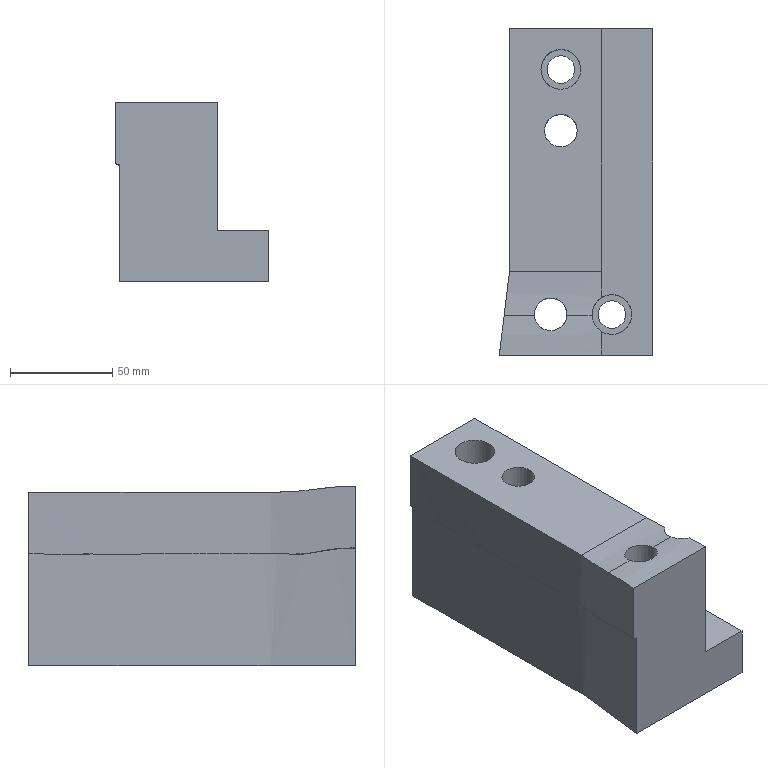Part | NX | features solid 2 | 1 solid | 21 faces | box 75.161 x 160 x 88.078 mm | volume 639767 mm3 | plane 9 | spline 6 | cylinder 6 | commonest cylinder face diameters 13.5 x2 16 x2 19.5 x2
STEP:
#1=CARTESIAN_POINT('',(-305.,78.37,-10.));
#2=VERTEX_POINT('',#1);
#3=CARTESIAN_POINT('',(-305.,78.37,50.536));
#4=VERTEX_POINT('',#3);
#5=CARTESIAN_POINT('',(-305.,78.37,-20.));
#6=DIRECTION('',(0.,0.,1.));
#7=VECTOR('',#6,1000.);
#8=LINE('',#5,#7);
#9=EDGE_CURVE('',#2,#4,#8,.T.);
#10=ORIENTED_EDGE('',*,*,#9,.F.);
#11=CARTESIAN_POINT('',(-305.,210.,-10.));
#12=VERTEX_POINT('',#11);
#13=CARTESIAN_POINT('',(-305.,315.,-10.));
#14=DIRECTION('',(0.,-1.,0.));
#15=VECTOR('',#14,1000.);
#16=LINE('',#13,#15);
#17=EDGE_CURVE('',#2,#12,#16,.F.);
#18=ORIENTED_EDGE('',*,*,#17,.T.);
#19=CARTESIAN_POINT('',(-305.,210.,50.));
#20=VERTEX_POINT('',#19);
#21=CARTESIAN_POINT('',(-305.,210.,-500.));
#22=DIRECTION('',(0.,0.,1.));
#23=VECTOR('',#22,1000.);
#24=LINE('',#21,#23);
#25=EDGE_CURVE('',#12,#20,#24,.T.);
#26=ORIENTED_EDGE('',*,*,#25,.T.);
#27=CARTESIAN_POINT('',(-305.,91.041,50.));
#28=VERTEX_POINT('',#27);
#29=CARTESIAN_POINT('',(-305.,91.041,50.));
#30=CARTESIAN_POINT('',(-305.,130.694,50.));
#31=CARTESIAN_POINT('',(-305.,170.347,50.));
#32=CARTESIAN_POINT('',(-305.,210.,50.));
#33=B_SPLINE_CURVE_WITH_KNOTS('',3,(#29,#30,#31,#32),.UNSPECIFIED.,.F.,.F.,(4,4),(0.,0.119),.UNSPECIFIED.);
#34=EDGE_CURVE('',#28,#20,#33,.T.);
#35=ORIENTED_EDGE('',*,*,#34,.F.);
#36=CARTESIAN_POINT('',(-305.,91.041,50.));
#37=CARTESIAN_POINT('',(-305.,86.812,50.));
#38=CARTESIAN_POINT('',(-305.,82.583,50.179));
#39=CARTESIAN_POINT('',(-305.,78.37,50.536));
#40=B_SPLINE_CURVE_WITH_KNOTS('',3,(#36,#37,#38,#39),.UNSPECIFIED.,.F.,.F.,(4,4),(0.,0.01269),.UNSPECIFIED.);
#41=EDGE_CURVE('',#28,#4,#40,.T.);
#42=ORIENTED_EDGE('',*,*,#41,.T.);
#43=EDGE_LOOP('',(#10,#18,#26,#35,#42));
#44=FACE_BOUND('',#43,.T.);
#45=CARTESIAN_POINT('',(-305.,340.,500.));
#46=DIRECTION('',(1.,0.,0.));
#47=DIRECTION('',(0.,0.,-1.));
#48=AXIS2_PLACEMENT_3D('',#45,#46,#47);
#49=PLANE('',#48);
#50=ADVANCED_FACE('',(#44),#49,.T.);
#51=CARTESIAN_POINT('',(-305.,61.63,52.478));
#52=VERTEX_POINT('',#51);
#53=CARTESIAN_POINT('',(-305.,61.63,-10.));
#54=VERTEX_POINT('',#53);
#55=CARTESIAN_POINT('',(-305.,61.63,-20.));
#56=DIRECTION('',(0.,0.,1.));
#57=VECTOR('',#56,1000.);
#58=LINE('',#55,#57);
#59=EDGE_CURVE('',#52,#54,#58,.F.);
#60=ORIENTED_EDGE('',*,*,#59,.F.);
#61=CARTESIAN_POINT('',(-305.,50.,53.078));
#62=VERTEX_POINT('',#61);
#63=CARTESIAN_POINT('',(-305.,50.,53.078));
#64=CARTESIAN_POINT('',(-305.,53.888,53.029));
#65=CARTESIAN_POINT('',(-305.,57.765,52.828));
#66=CARTESIAN_POINT('',(-305.,61.63,52.478));
#67=B_SPLINE_CURVE_WITH_KNOTS('',3,(#63,#64,#65,#66),.UNSPECIFIED.,.F.,.F.,(4,4),(0.,0.01164),.UNSPECIFIED.);
#68=EDGE_CURVE('',#62,#52,#67,.T.);
#69=ORIENTED_EDGE('',*,*,#68,.F.);
#70=CARTESIAN_POINT('',(-305.,50.,-10.));
#71=VERTEX_POINT('',#70);
#72=CARTESIAN_POINT('',(-305.,50.,-500.));
#73=DIRECTION('',(0.,0.,1.));
#74=VECTOR('',#73,1000.);
#75=LINE('',#72,#74);
#76=EDGE_CURVE('',#71,#62,#75,.T.);
#77=ORIENTED_EDGE('',*,*,#76,.F.);
#78=CARTESIAN_POINT('',(-305.,315.,-10.));
#79=DIRECTION('',(0.,-1.,0.));
#80=VECTOR('',#79,1000.);
#81=LINE('',#78,#80);
#82=EDGE_CURVE('',#71,#54,#81,.F.);
#83=ORIENTED_EDGE('',*,*,#82,.T.);
#84=EDGE_LOOP('',(#60,#69,#77,#83));
#85=FACE_BOUND('',#84,.T.);
#86=CARTESIAN_POINT('',(-305.,340.,500.));
#87=DIRECTION('',(1.,0.,0.));
#88=DIRECTION('',(0.,0.,-1.));
#89=AXIS2_PLACEMENT_3D('',#86,#87,#88);
#90=PLANE('',#89);
#91=ADVANCED_FACE('',(#85),#90,.T.);
#92=CARTESIAN_POINT('',(-353.138,50.,-35.));
#93=VERTEX_POINT('',#92);
#94=CARTESIAN_POINT('',(-280.,50.,-35.));
#95=VERTEX_POINT('',#94);
#96=CARTESIAN_POINT('',(-353.136,50.,-35.));
#97=DIRECTION('',(1.,0.,0.));
#98=VECTOR('',#97,1000.);
#99=LINE('',#96,#98);
#100=EDGE_CURVE('',#93,#95,#99,.T.);
#101=ORIENTED_EDGE('',*,*,#100,.T.);
#102=CARTESIAN_POINT('',(-280.,50.,-10.));
#103=VERTEX_POINT('',#102);
#104=CARTESIAN_POINT('',(-280.,50.,-500.));
#105=DIRECTION('',(0.,0.,1.));
#106=VECTOR('',#105,1000.);
#107=LINE('',#104,#106);
#108=EDGE_CURVE('',#95,#103,#107,.T.);
#109=ORIENTED_EDGE('',*,*,#108,.T.);
#110=CARTESIAN_POINT('',(365.,50.,-10.));
#111=DIRECTION('',(-1.,0.,0.));
#112=VECTOR('',#111,1000.);
#113=LINE('',#110,#112);
#114=EDGE_CURVE('',#71,#103,#113,.F.);
#115=ORIENTED_EDGE('',*,*,#114,.F.);
#116=ORIENTED_EDGE('',*,*,#76,.T.);
#117=CARTESIAN_POINT('',(-355.161,50.,53.078));
#118=VERTEX_POINT('',#117);
#119=CARTESIAN_POINT('',(-355.161,50.,53.078));
#120=CARTESIAN_POINT('',(-338.441,50.,53.078));
#121=CARTESIAN_POINT('',(-321.72,50.,53.078));
#122=CARTESIAN_POINT('',(-305.,50.,53.078));
#123=B_SPLINE_CURVE_WITH_KNOTS('',3,(#119,#120,#121,#122),.UNSPECIFIED.,.F.,.F.,(4,4),(0.00388,0.05404),.UNSPECIFIED.);
#124=EDGE_CURVE('',#118,#62,#123,.T.);
#125=ORIENTED_EDGE('',*,*,#124,.F.);
#126=CARTESIAN_POINT('',(-355.161,50.,22.792));
#127=VERTEX_POINT('',#126);
#128=CARTESIAN_POINT('',(-355.161,50.,37.356));
#129=DIRECTION('',(0.,0.,-1.));
#130=VECTOR('',#129,1000.);
#131=LINE('',#128,#130);
#132=EDGE_CURVE('',#118,#127,#131,.T.);
#133=ORIENTED_EDGE('',*,*,#132,.T.);
#134=CARTESIAN_POINT('',(-353.138,50.,22.67));
#135=VERTEX_POINT('',#134);
#136=CARTESIAN_POINT('',(-353.138,50.,22.67));
#137=CARTESIAN_POINT('',(-353.814,50.,22.701));
#138=CARTESIAN_POINT('',(-354.488,50.,22.741));
#139=CARTESIAN_POINT('',(-355.161,50.,22.792));
#140=B_SPLINE_CURVE_WITH_KNOTS('',3,(#136,#137,#138,#139),.UNSPECIFIED.,.F.,.F.,(4,4),(0.01465,0.01669),.UNSPECIFIED.);
#141=EDGE_CURVE('',#135,#127,#140,.T.);
#142=ORIENTED_EDGE('',*,*,#141,.F.);
#143=CARTESIAN_POINT('',(-353.138,50.,-84.379));
#144=DIRECTION('',(0.,0.,-1.));
#145=VECTOR('',#144,1000.);
#146=LINE('',#143,#145);
#147=EDGE_CURVE('',#93,#135,#146,.F.);
#148=ORIENTED_EDGE('',*,*,#147,.F.);
#149=EDGE_LOOP('',(#101,#109,#115,#116,#125,#133,#142,#148));
#150=FACE_BOUND('',#149,.T.);
#151=CARTESIAN_POINT('',(-353.136,50.,-500.));
#152=DIRECTION('',(0.,-1.,0.));
#153=DIRECTION('',(0.,0.,-1.));
#154=AXIS2_PLACEMENT_3D('',#151,#152,#153);
#155=PLANE('',#154);
#156=ADVANCED_FACE('',(#150),#155,.T.);
#157=ORIENTED_EDGE('',*,*,#25,.F.);
#158=CARTESIAN_POINT('',(-280.,210.,-10.));
#159=VERTEX_POINT('',#158);
#160=CARTESIAN_POINT('',(365.,210.,-10.));
#161=DIRECTION('',(-1.,0.,0.));
#162=VECTOR('',#161,1000.);
#163=LINE('',#160,#162);
#164=EDGE_CURVE('',#12,#159,#163,.F.);
#165=ORIENTED_EDGE('',*,*,#164,.T.);
#166=CARTESIAN_POINT('',(-280.,210.,-35.));
#167=VERTEX_POINT('',#166);
#168=CARTESIAN_POINT('',(-280.,210.,-500.));
#169=DIRECTION('',(0.,0.,1.));
#170=VECTOR('',#169,1000.);
#171=LINE('',#168,#170);
#172=EDGE_CURVE('',#167,#159,#171,.T.);
#173=ORIENTED_EDGE('',*,*,#172,.F.);
#174=CARTESIAN_POINT('',(-347.967,210.,-35.));
#175=VERTEX_POINT('',#174);
#176=CARTESIAN_POINT('',(-350.,210.,-35.));
#177=DIRECTION('',(1.,0.,0.));
#178=VECTOR('',#177,1000.);
#179=LINE('',#176,#178);
#180=EDGE_CURVE('',#175,#167,#179,.T.);
#181=ORIENTED_EDGE('',*,*,#180,.F.);
#182=CARTESIAN_POINT('',(-347.967,210.,19.922));
#183=VERTEX_POINT('',#182);
#184=CARTESIAN_POINT('',(-347.967,210.,-84.379));
#185=DIRECTION('',(0.,0.,-1.));
#186=VECTOR('',#185,1000.);
#187=LINE('',#184,#186);
#188=EDGE_CURVE('',#175,#183,#187,.F.);
#189=ORIENTED_EDGE('',*,*,#188,.T.);
#190=CARTESIAN_POINT('',(-349.967,210.,19.959));
#191=VERTEX_POINT('',#190);
#192=CARTESIAN_POINT('',(-347.967,210.,19.922));
#193=CARTESIAN_POINT('',(-348.633,210.,19.931));
#194=CARTESIAN_POINT('',(-349.3,210.,19.943));
#195=CARTESIAN_POINT('',(-349.967,210.,19.959));
#196=B_SPLINE_CURVE_WITH_KNOTS('',3,(#192,#193,#194,#195),.UNSPECIFIED.,.F.,.F.,(4,4),(0.004977,0.006977),.UNSPECIFIED.);
#197=EDGE_CURVE('',#183,#191,#196,.T.);
#198=ORIENTED_EDGE('',*,*,#197,.T.);
#199=CARTESIAN_POINT('',(-349.967,210.,50.));
#200=VERTEX_POINT('',#199);
#201=CARTESIAN_POINT('',(-349.967,210.,37.356));
#202=DIRECTION('',(0.,0.,-1.));
#203=VECTOR('',#202,1000.);
#204=LINE('',#201,#203);
#205=EDGE_CURVE('',#200,#191,#204,.T.);
#206=ORIENTED_EDGE('',*,*,#205,.F.);
#207=CARTESIAN_POINT('',(-265.,210.,50.));
#208=DIRECTION('',(1.,0.,0.));
#209=VECTOR('',#208,1000.);
#210=LINE('',#207,#209);
#211=EDGE_CURVE('',#200,#20,#210,.T.);
#212=ORIENTED_EDGE('',*,*,#211,.T.);
#213=EDGE_LOOP('',(#157,#165,#173,#181,#189,#198,#206,#212));
#214=FACE_BOUND('',#213,.T.);
#215=CARTESIAN_POINT('',(-350.,210.,-500.));
#216=DIRECTION('',(0.,-1.,0.));
#217=DIRECTION('',(0.,0.,-1.));
#218=AXIS2_PLACEMENT_3D('',#215,#216,#217);
#219=PLANE('',#218);
#220=ADVANCED_FACE('',(#214),#219,.F.);
#221=CARTESIAN_POINT('',(-337.988,69.567,51.545));
#222=VERTEX_POINT('',#221);
#223=CARTESIAN_POINT('',(-352.757,69.567,51.545));
#224=VERTEX_POINT('',#223);
#225=CARTESIAN_POINT('',(-337.988,69.567,51.545));
#226=CARTESIAN_POINT('',(-342.911,69.567,51.545));
#227=CARTESIAN_POINT('',(-347.834,69.567,51.545));
#228=CARTESIAN_POINT('',(-352.757,69.567,51.545));
#229=B_SPLINE_CURVE_WITH_KNOTS('',3,(#225,#226,#227,#228),.UNSPECIFIED.,.F.,.F.,(4,4),(0.9517,0.9933),.UNSPECIFIED.);
#230=EDGE_CURVE('',#222,#224,#229,.T.);
#231=ORIENTED_EDGE('',*,*,#230,.F.);
#232=CARTESIAN_POINT('',(-322.012,69.567,51.545));
#233=VERTEX_POINT('',#232);
#234=CARTESIAN_POINT('',(-337.988,69.567,51.545));
#235=CARTESIAN_POINT('',(-338.106,71.736,51.231));
#236=CARTESIAN_POINT('',(-336.503,76.106,50.718));
#237=CARTESIAN_POINT('',(-330.012,78.945,50.493));
#238=CARTESIAN_POINT('',(-323.498,76.115,50.717));
#239=CARTESIAN_POINT('',(-321.894,71.736,51.231));
#240=CARTESIAN_POINT('',(-322.012,69.567,51.545));
#241=B_SPLINE_CURVE_WITH_KNOTS('',3,(#234,#235,#236,#237,#238,#239,#240),.UNSPECIFIED.,.F.,.F.,(4,1,1,1,4),(0.,0.006491,0.01298,0.01947,0.02596),.UNSPECIFIED.);
#242=EDGE_CURVE('',#222,#233,#241,.T.);
#243=ORIENTED_EDGE('',*,*,#242,.T.);
#244=CARTESIAN_POINT('',(-309.74,69.567,51.545));
#245=VERTEX_POINT('',#244);
#246=CARTESIAN_POINT('',(-309.74,69.567,51.545));
#247=CARTESIAN_POINT('',(-313.831,69.567,51.545));
#248=CARTESIAN_POINT('',(-317.921,69.567,51.545));
#249=CARTESIAN_POINT('',(-322.012,69.567,51.545));
#250=B_SPLINE_CURVE_WITH_KNOTS('',3,(#246,#247,#248,#249),.UNSPECIFIED.,.F.,.F.,(4,4),(0.8721,0.9067),.UNSPECIFIED.);
#251=EDGE_CURVE('',#245,#233,#250,.T.);
#252=ORIENTED_EDGE('',*,*,#251,.F.);
#253=CARTESIAN_POINT('',(-309.74,69.567,51.545));
#254=CARTESIAN_POINT('',(-309.896,73.076,51.038));
#255=CARTESIAN_POINT('',(-308.044,76.552,50.69));
#256=CARTESIAN_POINT('',(-305.,78.37,50.536));
#257=B_SPLINE_CURVE_WITH_KNOTS('',3,(#253,#254,#255,#256),.UNSPECIFIED.,.F.,.F.,(4,4),(0.,0.0105),.UNSPECIFIED.);
#258=EDGE_CURVE('',#245,#4,#257,.T.);
#259=ORIENTED_EDGE('',*,*,#258,.T.);
#260=ORIENTED_EDGE('',*,*,#41,.F.);
#261=CARTESIAN_POINT('',(-350.144,91.041,50.));
#262=VERTEX_POINT('',#261);
#263=CARTESIAN_POINT('',(-350.144,91.041,50.));
#264=CARTESIAN_POINT('',(-335.096,91.041,50.));
#265=CARTESIAN_POINT('',(-320.048,91.041,50.));
#266=CARTESIAN_POINT('',(-305.,91.041,50.));
#267=B_SPLINE_CURVE_WITH_KNOTS('',3,(#263,#264,#265,#266),.UNSPECIFIED.,.F.,.F.,(4,4),(0.03072,0.3146),.UNSPECIFIED.);
#268=EDGE_CURVE('',#262,#28,#267,.T.);
#269=ORIENTED_EDGE('',*,*,#268,.F.);
#270=CARTESIAN_POINT('',(-350.144,91.041,50.));
#271=CARTESIAN_POINT('',(-350.286,89.236,50.));
#272=CARTESIAN_POINT('',(-350.787,85.654,50.065));
#273=CARTESIAN_POINT('',(-351.671,78.483,50.451));
#274=CARTESIAN_POINT('',(-352.321,73.122,51.031));
#275=CARTESIAN_POINT('',(-352.757,69.567,51.545));
#276=B_SPLINE_CURVE_WITH_KNOTS('',3,(#270,#271,#272,#273,#274,#275),.UNSPECIFIED.,.F.,.F.,(4,1,1,4),(0.,0.005425,0.01085,0.0217),.UNSPECIFIED.);
#277=EDGE_CURVE('',#262,#224,#276,.T.);
#278=ORIENTED_EDGE('',*,*,#277,.T.);
#279=EDGE_LOOP('',(#231,#243,#252,#259,#260,#269,#278));
#280=FACE_BOUND('',#279,.T.);
#281=CARTESIAN_POINT('',(-305.,69.567,51.545));
#282=CARTESIAN_POINT('',(-305.,80.248,50.));
#283=CARTESIAN_POINT('',(-305.,91.041,50.));
#284=CARTESIAN_POINT('',(-321.014,69.567,51.545));
#285=CARTESIAN_POINT('',(-321.014,80.248,50.));
#286=CARTESIAN_POINT('',(-321.014,91.041,50.));
#287=CARTESIAN_POINT('',(-337.029,69.567,51.545));
#288=CARTESIAN_POINT('',(-337.029,80.248,50.));
#289=CARTESIAN_POINT('',(-337.029,91.041,50.));
#290=CARTESIAN_POINT('',(-353.043,69.567,51.545));
#291=CARTESIAN_POINT('',(-353.043,80.248,50.));
#292=CARTESIAN_POINT('',(-353.043,91.041,50.));
#293=(BOUNDED_SURFACE()B_SPLINE_SURFACE(3,2,((#281,#282,#283),(#284,#285,#286),(#287,#288,#289),(#290,#291,#292)),.UNSPECIFIED.,.F.,.F.,.F.)B_SPLINE_SURFACE_WITH_KNOTS((4,4),(3,3),(0.8537,0.9881),(0.,1.),.PIECEWISE_BEZIER_KNOTS.)GEOMETRIC_REPRESENTATION_ITEM()RATIONAL_B_SPLINE_SURFACE(((1.,0.9974,1.),(1.,0.9974,1.),(1.,0.9974,1.),(1.,0.9974,1.)))REPRESENTATION_ITEM('')SURFACE());
#294=ADVANCED_FACE('',(#280),#293,.F.);
#295=CARTESIAN_POINT('',(-317.,160.,50.));
#296=VERTEX_POINT('',#295);
#297=CARTESIAN_POINT('',(-318.736,153.724,50.));
#298=CARTESIAN_POINT('',(-316.133,160.002,50.));
#299=CARTESIAN_POINT('',(-318.734,166.27,50.));
#300=CARTESIAN_POINT('',(-324.994,168.864,50.));
#301=CARTESIAN_POINT('',(-331.266,166.273,50.));
#302=CARTESIAN_POINT('',(-333.865,160.001,50.));
#303=CARTESIAN_POINT('',(-331.275,153.739,50.));
#304=CARTESIAN_POINT('',(-325.01,151.134,50.));
#305=CARTESIAN_POINT('',(-318.736,153.724,50.));
#306=CARTESIAN_POINT('',(-316.133,160.002,50.));
#307=CARTESIAN_POINT('',(-318.734,166.27,50.));
#308=B_SPLINE_CURVE_WITH_KNOTS('',3,(#297,#298,#299,#300,#301,#302,#303,#304,#305,#306,#307),.UNSPECIFIED.,.T.,.F.,(1,1,1,1,1,1,1,1,1,1,1,1,1,1,1),(-0.01876,-0.0125,-0.006252,0.,0.006252,0.0125,0.01876,0.02501,0.03126,0.03751,0.04377,0.05002,0.05627,0.06252,0.06877),.UNSPECIFIED.);
#309=EDGE_CURVE('',#296,#296,#308,.T.);
#310=ORIENTED_EDGE('',*,*,#309,.F.);
#311=EDGE_LOOP('',(#310));
#312=FACE_BOUND('',#311,.T.);
#313=CARTESIAN_POINT('',(-315.25,190.,50.));
#314=VERTEX_POINT('',#313);
#315=CARTESIAN_POINT('',(-317.366,182.351,50.));
#316=CARTESIAN_POINT('',(-314.193,190.002,50.));
#317=CARTESIAN_POINT('',(-317.363,197.641,50.));
#318=CARTESIAN_POINT('',(-324.992,200.803,50.));
#319=CARTESIAN_POINT('',(-332.637,197.646,50.));
#320=CARTESIAN_POINT('',(-335.804,190.001,50.));
#321=CARTESIAN_POINT('',(-332.648,182.37,50.));
#322=CARTESIAN_POINT('',(-325.012,179.195,50.));
#323=CARTESIAN_POINT('',(-317.366,182.351,50.));
#324=CARTESIAN_POINT('',(-314.193,190.002,50.));
#325=CARTESIAN_POINT('',(-317.363,197.641,50.));
#326=B_SPLINE_CURVE_WITH_KNOTS('',3,(#315,#316,#317,#318,#319,#320,#321,#322,#323,#324,#325),.UNSPECIFIED.,.T.,.F.,(1,1,1,1,1,1,1,1,1,1,1,1,1,1,1),(-0.02286,-0.01524,-0.00762,0.,0.00762,0.01524,0.02286,0.03048,0.0381,0.04572,0.05334,0.06096,0.06858,0.0762,0.08382),.UNSPECIFIED.);
#327=EDGE_CURVE('',#314,#314,#326,.T.);
#328=ORIENTED_EDGE('',*,*,#327,.F.);
#329=EDGE_LOOP('',(#328));
#330=FACE_BOUND('',#329,.T.);
#331=ORIENTED_EDGE('',*,*,#268,.T.);
#332=ORIENTED_EDGE('',*,*,#34,.T.);
#333=ORIENTED_EDGE('',*,*,#211,.F.);
#334=CARTESIAN_POINT('',(-350.144,91.041,50.));
#335=CARTESIAN_POINT('',(-349.948,93.519,50.));
#336=CARTESIAN_POINT('',(-350.035,98.476,50.));
#337=CARTESIAN_POINT('',(-350.015,105.911,50.));
#338=CARTESIAN_POINT('',(-350.022,113.346,50.));
#339=CARTESIAN_POINT('',(-350.007,123.259,50.));
#340=CARTESIAN_POINT('',(-350.002,135.65,50.));
#341=CARTESIAN_POINT('',(-349.996,155.476,50.));
#342=CARTESIAN_POINT('',(-350.034,180.259,50.));
#343=CARTESIAN_POINT('',(-349.982,200.087,50.));
#344=CARTESIAN_POINT('',(-349.967,210.,50.));
#345=B_SPLINE_CURVE_WITH_KNOTS('',3,(#334,#335,#336,#337,#338,#339,#340,#341,#342,#343,#344),.UNSPECIFIED.,.F.,.F.,(4,1,1,1,1,1,1,1,4),(0.,0.007435,0.01487,0.0223,0.02974,0.04461,0.05948,0.08922,0.119),.UNSPECIFIED.);
#346=EDGE_CURVE('',#262,#200,#345,.T.);
#347=ORIENTED_EDGE('',*,*,#346,.F.);
#348=EDGE_LOOP('',(#331,#332,#333,#347));
#349=FACE_BOUND('',#348,.T.);
#350=CARTESIAN_POINT('',(-305.,91.041,50.));
#351=CARTESIAN_POINT('',(-350.415,91.041,50.));
#352=CARTESIAN_POINT('',(-305.,210.,50.));
#353=CARTESIAN_POINT('',(-350.415,210.,50.));
#354=B_SPLINE_SURFACE_WITH_KNOTS('',1,1,((#350,#351),(#352,#353)),.PLANE_SURF.,.F.,.F.,.F.,(2,2),(2,2),(0.,0.471),(0.5755,0.6612),.PIECEWISE_BEZIER_KNOTS.);
#355=ADVANCED_FACE('',(#312,#330,#349),#354,.T.);
#356=CARTESIAN_POINT('',(-337.988,69.567,51.545));
#357=CARTESIAN_POINT('',(-337.878,67.542,51.838));
#358=CARTESIAN_POINT('',(-336.073,63.634,52.304));
#359=CARTESIAN_POINT('',(-330.001,61.184,52.514));
#360=CARTESIAN_POINT('',(-323.928,63.632,52.304));
#361=CARTESIAN_POINT('',(-322.122,67.542,51.838));
#362=CARTESIAN_POINT('',(-322.012,69.567,51.545));
#363=B_SPLINE_CURVE_WITH_KNOTS('',3,(#356,#357,#358,#359,#360,#361,#362),.UNSPECIFIED.,.F.,.F.,(4,1,1,1,4),(0.,0.00606,0.01212,0.01818,0.02424),.UNSPECIFIED.);
#364=EDGE_CURVE('',#222,#233,#363,.T.);
#365=ORIENTED_EDGE('',*,*,#364,.F.);
#366=ORIENTED_EDGE('',*,*,#230,.T.);
#367=CARTESIAN_POINT('',(-355.161,50.,53.078));
#368=CARTESIAN_POINT('',(-354.357,56.548,52.995));
#369=CARTESIAN_POINT('',(-353.553,63.081,52.483));
#370=CARTESIAN_POINT('',(-352.757,69.567,51.545));
#371=B_SPLINE_CURVE_WITH_KNOTS('',3,(#367,#368,#369,#370),.UNSPECIFIED.,.F.,.F.,(4,4),(0.02067,0.04046),.UNSPECIFIED.);
#372=EDGE_CURVE('',#118,#224,#371,.T.);
#373=ORIENTED_EDGE('',*,*,#372,.F.);
#374=ORIENTED_EDGE('',*,*,#124,.T.);
#375=ORIENTED_EDGE('',*,*,#68,.T.);
#376=CARTESIAN_POINT('',(-309.74,69.567,51.545));
#377=CARTESIAN_POINT('',(-309.597,66.347,52.011));
#378=CARTESIAN_POINT('',(-307.793,63.298,52.327));
#379=CARTESIAN_POINT('',(-305.,61.63,52.478));
#380=B_SPLINE_CURVE_WITH_KNOTS('',3,(#376,#377,#378,#379),.UNSPECIFIED.,.F.,.F.,(4,4),(0.,0.009631),.UNSPECIFIED.);
#381=EDGE_CURVE('',#245,#52,#380,.T.);
#382=ORIENTED_EDGE('',*,*,#381,.F.);
#383=ORIENTED_EDGE('',*,*,#251,.T.);
#384=EDGE_LOOP('',(#365,#366,#373,#374,#375,#382,#383));
#385=FACE_BOUND('',#384,.T.);
#386=CARTESIAN_POINT('',(-305.,69.567,51.545));
#387=CARTESIAN_POINT('',(-305.,59.775,52.962));
#388=CARTESIAN_POINT('',(-305.,49.882,53.08));
#389=CARTESIAN_POINT('',(-321.821,69.567,51.545));
#390=CARTESIAN_POINT('',(-321.821,59.775,52.962));
#391=CARTESIAN_POINT('',(-321.821,49.882,53.08));
#392=CARTESIAN_POINT('',(-338.641,69.567,51.545));
#393=CARTESIAN_POINT('',(-338.641,59.775,52.962));
#394=CARTESIAN_POINT('',(-338.641,49.882,53.08));
#395=CARTESIAN_POINT('',(-355.462,69.567,51.545));
#396=CARTESIAN_POINT('',(-355.462,59.775,52.962));
#397=CARTESIAN_POINT('',(-355.462,49.882,53.08));
#398=(BOUNDED_SURFACE()B_SPLINE_SURFACE(3,2,((#386,#387,#388),(#389,#390,#391),(#392,#393,#394),(#395,#396,#397)),.UNSPECIFIED.,.F.,.F.,.F.)B_SPLINE_SURFACE_WITH_KNOTS((4,4),(3,3),(0.3833,0.4467),(0.1505,0.5681),.PIECEWISE_BEZIER_KNOTS.)GEOMETRIC_REPRESENTATION_ITEM()RATIONAL_B_SPLINE_SURFACE(((0.9968,0.9932,0.9939),(0.9968,0.9932,0.9939),(0.9968,0.9932,0.9939),(0.9968,0.9932,0.9939)))REPRESENTATION_ITEM('')SURFACE());
#399=ADVANCED_FACE('',(#385),#398,.T.);
#400=CARTESIAN_POINT('',(-338.,70.,-35.));
#401=VERTEX_POINT('',#400);
#402=CARTESIAN_POINT('',(-330.,70.,-35.));
#403=DIRECTION('',(0.,0.,-1.));
#404=DIRECTION('',(-1.,0.,0.));
#405=AXIS2_PLACEMENT_3D('',#402,#403,#404);
#406=CIRCLE('',#405,8.);
#407=EDGE_CURVE('',#401,#401,#406,.T.);
#408=ORIENTED_EDGE('',*,*,#407,.F.);
#409=EDGE_LOOP('',(#408));
#410=FACE_BOUND('',#409,.T.);
#411=CARTESIAN_POINT('',(-333.,160.,-35.));
#412=VERTEX_POINT('',#411);
#413=CARTESIAN_POINT('',(-325.,160.,-35.));
#414=DIRECTION('',(0.,0.,-1.));
#415=DIRECTION('',(-1.,0.,0.));
#416=AXIS2_PLACEMENT_3D('',#413,#414,#415);
#417=CIRCLE('',#416,8.);
#418=EDGE_CURVE('',#412,#412,#417,.T.);
#419=ORIENTED_EDGE('',*,*,#418,.F.);
#420=EDGE_LOOP('',(#419));
#421=FACE_BOUND('',#420,.T.);
#422=CARTESIAN_POINT('',(-331.75,190.,-35.));
#423=VERTEX_POINT('',#422);
#424=CARTESIAN_POINT('',(-325.,190.,-35.));
#425=DIRECTION('',(0.,0.,-1.));
#426=DIRECTION('',(-1.,0.,0.));
#427=AXIS2_PLACEMENT_3D('',#424,#425,#426);
#428=CIRCLE('',#427,6.75);
#429=EDGE_CURVE('',#423,#423,#428,.T.);
#430=ORIENTED_EDGE('',*,*,#429,.F.);
#431=EDGE_LOOP('',(#430));
#432=FACE_BOUND('',#431,.T.);
#433=CARTESIAN_POINT('',(-306.75,70.,-35.));
#434=VERTEX_POINT('',#433);
#435=CARTESIAN_POINT('',(-300.,70.,-35.));
#436=DIRECTION('',(0.,0.,-1.));
#437=DIRECTION('',(-1.,0.,0.));
#438=AXIS2_PLACEMENT_3D('',#435,#436,#437);
#439=CIRCLE('',#438,6.75);
#440=EDGE_CURVE('',#434,#434,#439,.T.);
#441=ORIENTED_EDGE('',*,*,#440,.F.);
#442=EDGE_LOOP('',(#441));
#443=FACE_BOUND('',#442,.T.);
#444=ORIENTED_EDGE('',*,*,#180,.T.);
#445=CARTESIAN_POINT('',(-280.,210.,-35.));
#446=DIRECTION('',(0.,1.,0.));
#447=VECTOR('',#446,1000.);
#448=LINE('',#445,#447);
#449=EDGE_CURVE('',#95,#167,#448,.T.);
#450=ORIENTED_EDGE('',*,*,#449,.F.);
#451=ORIENTED_EDGE('',*,*,#100,.F.);
#452=CARTESIAN_POINT('',(-347.967,210.,-35.));
#453=CARTESIAN_POINT('',(-348.054,196.644,-35.));
#454=CARTESIAN_POINT('',(-348.021,176.61,-35.));
#455=CARTESIAN_POINT('',(-348.017,149.897,-35.));
#456=CARTESIAN_POINT('',(-348.014,133.202,-35.));
#457=CARTESIAN_POINT('',(-348.004,119.846,-35.));
#458=CARTESIAN_POINT('',(-347.996,109.829,-35.));
#459=CARTESIAN_POINT('',(-348.008,101.482,-35.));
#460=CARTESIAN_POINT('',(-347.966,94.802,-35.));
#461=CARTESIAN_POINT('',(-348.187,89.805,-35.));
#462=CARTESIAN_POINT('',(-348.853,84.832,-35.));
#463=CARTESIAN_POINT('',(-349.703,78.199,-35.));
#464=CARTESIAN_POINT('',(-350.707,69.905,-35.));
#465=CARTESIAN_POINT('',(-351.92,59.952,-35.));
#466=CARTESIAN_POINT('',(-352.73,53.317,-35.));
#467=CARTESIAN_POINT('',(-353.138,50.,-35.));
#468=B_SPLINE_CURVE_WITH_KNOTS('',3,(#452,#453,#454,#455,#456,#457,#458,#459,#460,#461,#462,#463,#464,#465,#466,#467),.UNSPECIFIED.,.F.,.F.,(4,1,1,1,1,1,1,1,1,1,1,1,1,4),(0.,0.04007,0.0601,0.08014,0.09015,0.1002,0.1102,0.1152,0.1202,0.1252,0.1302,0.1402,0.1503,0.1603),.UNSPECIFIED.);
#469=EDGE_CURVE('',#175,#93,#468,.T.);
#470=ORIENTED_EDGE('',*,*,#469,.F.);
#471=EDGE_LOOP('',(#444,#450,#451,#470));
#472=FACE_BOUND('',#471,.T.);
#473=CARTESIAN_POINT('',(-1052.904,47.5,-35.));
#474=DIRECTION('',(0.,0.,-1.));
#475=DIRECTION('',(-1.,0.,0.));
#476=AXIS2_PLACEMENT_3D('',#473,#474,#475);
#477=PLANE('',#476);
#478=ADVANCED_FACE('',(#410,#421,#432,#443,#472),#477,.T.);
#479=ORIENTED_EDGE('',*,*,#188,.F.);
#480=ORIENTED_EDGE('',*,*,#469,.T.);
#481=ORIENTED_EDGE('',*,*,#147,.T.);
#482=CARTESIAN_POINT('',(-353.138,50.,22.67));
#483=CARTESIAN_POINT('',(-352.732,53.305,22.639));
#484=CARTESIAN_POINT('',(-352.127,58.258,22.445));
#485=CARTESIAN_POINT('',(-351.323,64.843,21.57));
#486=CARTESIAN_POINT('',(-350.725,69.771,20.559));
#487=CARTESIAN_POINT('',(-350.127,74.704,19.729));
#488=CARTESIAN_POINT('',(-349.516,79.66,19.634));
#489=CARTESIAN_POINT('',(-348.878,84.632,20.13));
#490=CARTESIAN_POINT('',(-348.214,89.585,20.166));
#491=CARTESIAN_POINT('',(-347.962,94.579,19.869));
#492=CARTESIAN_POINT('',(-348.002,99.604,19.878));
#493=CARTESIAN_POINT('',(-347.989,104.621,19.953));
#494=CARTESIAN_POINT('',(-348.005,111.312,19.885));
#495=CARTESIAN_POINT('',(-348.001,119.675,19.809));
#496=CARTESIAN_POINT('',(-348.013,129.712,19.927));
#497=CARTESIAN_POINT('',(-348.013,138.076,19.876));
#498=CARTESIAN_POINT('',(-348.016,144.767,19.874));
#499=CARTESIAN_POINT('',(-348.017,149.785,19.953));
#500=CARTESIAN_POINT('',(-348.018,154.804,20.028));
#501=CARTESIAN_POINT('',(-348.019,159.821,19.701));
#502=CARTESIAN_POINT('',(-348.021,164.838,19.316));
#503=CARTESIAN_POINT('',(-348.024,169.857,19.556));
#504=CARTESIAN_POINT('',(-348.025,174.876,19.851));
#505=CARTESIAN_POINT('',(-348.024,181.567,19.886));
#506=CARTESIAN_POINT('',(-348.025,188.257,19.693));
#507=CARTESIAN_POINT('',(-348.018,194.949,19.558));
#508=CARTESIAN_POINT('',(-348.004,201.637,19.831));
#509=CARTESIAN_POINT('',(-347.989,206.654,19.929));
#510=CARTESIAN_POINT('',(-347.967,210.,19.922));
#511=B_SPLINE_CURVE_WITH_KNOTS('',3,(#482,#483,#484,#485,#486,#487,#488,#489,#490,#491,#492,#493,#494,#495,#496,#497,#498,#499,#500,#501,#502,#503,#504,#505,#506,#507,#508,#509,#510),.UNSPECIFIED.,.F.,.F.,(4,1,1,1,1,1,1,1,1,1,1,1,1,1,1,1,1,1,1,1,1,1,1,1,1,1,4),(0.2882,0.298,0.3028,0.3077,0.3126,0.3174,0.3223,0.3272,0.332,0.3369,0.3418,0.3467,0.3564,0.3661,0.3759,0.3807,0.3856,0.3905,0.3954,0.4002,0.4051,0.41,0.4148,0.4246,0.4294,0.4343,0.4441),.UNSPECIFIED.);
#512=EDGE_CURVE('',#135,#183,#511,.T.);
#513=ORIENTED_EDGE('',*,*,#512,.T.);
#514=EDGE_LOOP('',(#479,#480,#481,#513));
#515=FACE_BOUND('',#514,.T.);
#516=CARTESIAN_POINT('',(-353.138,50.,23.016));
#517=CARTESIAN_POINT('',(-353.138,50.,-35.));
#518=CARTESIAN_POINT('',(-352.73,53.315,23.016));
#519=CARTESIAN_POINT('',(-352.73,53.315,-35.));
#520=CARTESIAN_POINT('',(-351.921,59.945,23.016));
#521=CARTESIAN_POINT('',(-351.921,59.945,-35.));
#522=CARTESIAN_POINT('',(-350.709,69.89,23.016));
#523=CARTESIAN_POINT('',(-350.709,69.89,-35.));
#524=CARTESIAN_POINT('',(-349.705,78.18,23.016));
#525=CARTESIAN_POINT('',(-349.705,78.18,-35.));
#526=CARTESIAN_POINT('',(-348.857,84.804,23.016));
#527=CARTESIAN_POINT('',(-348.857,84.804,-35.));
#528=CARTESIAN_POINT('',(-348.191,89.773,23.016));
#529=CARTESIAN_POINT('',(-348.191,89.773,-35.));
#530=CARTESIAN_POINT('',(-347.966,94.779,23.016));
#531=CARTESIAN_POINT('',(-347.966,94.779,-35.));
#532=CARTESIAN_POINT('',(-348.008,101.459,23.016));
#533=CARTESIAN_POINT('',(-348.008,101.459,-35.));
#534=CARTESIAN_POINT('',(-347.996,109.808,23.016));
#535=CARTESIAN_POINT('',(-347.996,109.808,-35.));
#536=CARTESIAN_POINT('',(-348.004,119.828,23.016));
#537=CARTESIAN_POINT('',(-348.004,119.828,-35.));
#538=CARTESIAN_POINT('',(-348.014,133.186,23.016));
#539=CARTESIAN_POINT('',(-348.014,133.186,-35.));
#540=CARTESIAN_POINT('',(-348.017,149.885,23.016));
#541=CARTESIAN_POINT('',(-348.017,149.885,-35.));
#542=CARTESIAN_POINT('',(-348.021,176.603,23.016));
#543=CARTESIAN_POINT('',(-348.021,176.603,-35.));
#544=CARTESIAN_POINT('',(-348.054,196.642,23.016));
#545=CARTESIAN_POINT('',(-348.054,196.642,-35.));
#546=CARTESIAN_POINT('',(-347.967,210.,23.016));
#547=CARTESIAN_POINT('',(-347.967,210.,-35.));
#548=B_SPLINE_SURFACE_WITH_KNOTS('',3,1,((#516,#517),(#518,#519),(#520,#521),(#522,#523),(#524,#525),(#526,#527),(#528,#529),(#530,#531),(#532,#533),(#534,#535),(#536,#537),(#538,#539),(#540,#541),(#542,#543),(#544,#545),(#546,#547)),.SURF_OF_LINEAR_EXTRUSION.,.F.,.F.,.F.,(4,1,1,1,1,1,1,1,1,1,1,1,1,4),(2,2),(0.7967,0.8069,0.817,0.8272,0.8322,0.8373,0.8424,0.8474,0.8576,0.8677,0.8778,0.8981,0.9184,0.9589),(0.,1.),.UNSPECIFIED.);
#549=ADVANCED_FACE('',(#515),#548,.T.);
#550=ORIENTED_EDGE('',*,*,#132,.F.);
#551=ORIENTED_EDGE('',*,*,#372,.T.);
#552=ORIENTED_EDGE('',*,*,#277,.F.);
#553=ORIENTED_EDGE('',*,*,#346,.T.);
#554=ORIENTED_EDGE('',*,*,#205,.T.);
#555=CARTESIAN_POINT('',(-349.967,210.,19.959));
#556=CARTESIAN_POINT('',(-349.969,208.333,19.965));
#557=CARTESIAN_POINT('',(-349.992,204.997,19.926));
#558=CARTESIAN_POINT('',(-350.011,199.995,19.711));
#559=CARTESIAN_POINT('',(-350.015,194.993,19.442));
#560=CARTESIAN_POINT('',(-350.034,188.322,19.647));
#561=CARTESIAN_POINT('',(-350.013,181.653,19.901));
#562=CARTESIAN_POINT('',(-350.008,174.982,19.844));
#563=CARTESIAN_POINT('',(-350.005,169.976,19.498));
#564=CARTESIAN_POINT('',(-350.002,164.972,19.216));
#565=CARTESIAN_POINT('',(-350.,159.971,19.651));
#566=CARTESIAN_POINT('',(-350.001,154.97,20.056));
#567=CARTESIAN_POINT('',(-350.001,149.967,19.988));
#568=CARTESIAN_POINT('',(-350.001,144.963,19.901));
#569=CARTESIAN_POINT('',(-350.002,138.291,19.911));
#570=CARTESIAN_POINT('',(-350.006,129.951,19.937));
#571=CARTESIAN_POINT('',(-350.01,119.944,19.798));
#572=CARTESIAN_POINT('',(-350.026,111.604,19.884));
#573=CARTESIAN_POINT('',(-350.016,104.932,19.959));
#574=CARTESIAN_POINT('',(-350.023,99.929,19.914));
#575=CARTESIAN_POINT('',(-349.962,94.923,19.886));
#576=CARTESIAN_POINT('',(-350.158,89.924,20.159));
#577=CARTESIAN_POINT('',(-350.884,84.94,20.077));
#578=CARTESIAN_POINT('',(-351.485,79.953,19.558));
#579=CARTESIAN_POINT('',(-352.106,74.97,19.697));
#580=CARTESIAN_POINT('',(-352.705,69.964,20.637));
#581=CARTESIAN_POINT('',(-353.325,64.952,21.698));
#582=CARTESIAN_POINT('',(-354.143,58.291,22.59));
#583=CARTESIAN_POINT('',(-354.754,53.314,22.772));
#584=CARTESIAN_POINT('',(-355.161,50.,22.792));
#585=B_SPLINE_CURVE_WITH_KNOTS('',3,(#555,#556,#557,#558,#559,#560,#561,#562,#563,#564,#565,#566,#567,#568,#569,#570,#571,#572,#573,#574,#575,#576,#577,#578,#579,#580,#581,#582,#583,#584),.UNSPECIFIED.,.F.,.F.,(4,1,1,1,1,1,1,1,1,1,1,1,1,1,1,1,1,1,1,1,1,1,1,1,1,1,1,4),(0.03871,0.04377,0.04883,0.05389,0.05895,0.06906,0.07412,0.07918,0.08424,0.0893,0.09436,0.09942,0.1045,0.1095,0.1197,0.1298,0.1399,0.1449,0.15,0.1551,0.1601,0.1652,0.1702,0.1753,0.1804,0.1854,0.1905,0.2006),.UNSPECIFIED.);
#586=EDGE_CURVE('',#191,#127,#585,.T.);
#587=ORIENTED_EDGE('',*,*,#586,.T.);
#588=EDGE_LOOP('',(#550,#551,#552,#553,#554,#587));
#589=FACE_BOUND('',#588,.T.);
#590=CARTESIAN_POINT('',(-349.967,210.,53.292));
#591=CARTESIAN_POINT('',(-349.967,210.,17.229));
#592=CARTESIAN_POINT('',(-349.977,203.321,53.292));
#593=CARTESIAN_POINT('',(-349.977,203.321,17.229));
#594=CARTESIAN_POINT('',(-350.056,189.961,53.292));
#595=CARTESIAN_POINT('',(-350.056,189.961,17.229));
#596=CARTESIAN_POINT('',(-349.993,169.923,53.292));
#597=CARTESIAN_POINT('',(-349.993,169.923,17.229));
#598=CARTESIAN_POINT('',(-350.003,149.884,53.292));
#599=CARTESIAN_POINT('',(-350.003,149.884,17.229));
#600=CARTESIAN_POINT('',(-350.002,133.185,53.292));
#601=CARTESIAN_POINT('',(-350.002,133.185,17.229));
#602=CARTESIAN_POINT('',(-350.013,119.826,53.292));
#603=CARTESIAN_POINT('',(-350.013,119.826,17.229));
#604=CARTESIAN_POINT('',(-350.018,109.806,53.292));
#605=CARTESIAN_POINT('',(-350.018,109.806,17.229));
#606=CARTESIAN_POINT('',(-350.04,101.457,53.292));
#607=CARTESIAN_POINT('',(-350.04,101.457,17.229));
#608=CARTESIAN_POINT('',(-349.959,94.777,53.292));
#609=CARTESIAN_POINT('',(-349.959,94.777,17.229));
#610=CARTESIAN_POINT('',(-350.178,89.77,53.292));
#611=CARTESIAN_POINT('',(-350.178,89.77,17.229));
#612=CARTESIAN_POINT('',(-350.9,84.807,53.292));
#613=CARTESIAN_POINT('',(-350.9,84.807,17.229));
#614=CARTESIAN_POINT('',(-351.704,78.177,53.292));
#615=CARTESIAN_POINT('',(-351.704,78.177,17.229));
#616=CARTESIAN_POINT('',(-352.716,69.889,53.292));
#617=CARTESIAN_POINT('',(-352.716,69.889,17.229));
#618=CARTESIAN_POINT('',(-353.94,59.945,53.292));
#619=CARTESIAN_POINT('',(-353.94,59.945,17.229));
#620=CARTESIAN_POINT('',(-354.754,53.315,53.292));
#621=CARTESIAN_POINT('',(-354.754,53.315,17.229));
#622=CARTESIAN_POINT('',(-355.161,50.,53.292));
#623=CARTESIAN_POINT('',(-355.161,50.,17.229));
#624=B_SPLINE_SURFACE_WITH_KNOTS('',3,1,((#590,#591),(#592,#593),(#594,#595),(#596,#597),(#598,#599),(#600,#601),(#602,#603),(#604,#605),(#606,#607),(#608,#609),(#610,#611),(#612,#613),(#614,#615),(#616,#617),(#618,#619),(#620,#621),(#622,#623)),.SURF_OF_LINEAR_EXTRUSION.,.F.,.F.,.F.,(4,1,1,1,1,1,1,1,1,1,1,1,1,1,4),(2,2),(0.5393,0.5599,0.5804,0.6009,0.6214,0.6317,0.642,0.6522,0.6574,0.6625,0.6676,0.6728,0.683,0.6933,0.7035),(0.,1.),.UNSPECIFIED.);
#625=ADVANCED_FACE('',(#589),#624,.F.);
#626=ORIENTED_EDGE('',*,*,#512,.F.);
#627=ORIENTED_EDGE('',*,*,#141,.T.);
#628=ORIENTED_EDGE('',*,*,#586,.F.);
#629=ORIENTED_EDGE('',*,*,#197,.F.);
#630=EDGE_LOOP('',(#626,#627,#628,#629));
#631=FACE_BOUND('',#630,.T.);
#632=CARTESIAN_POINT('',(-354.935,210.,20.15));
#633=CARTESIAN_POINT('',(-355.887,208.109,20.215));
#634=CARTESIAN_POINT('',(-358.002,203.344,20.282));
#635=CARTESIAN_POINT('',(-355.451,195.539,19.285));
#636=CARTESIAN_POINT('',(-357.141,185.362,20.216));
#637=CARTESIAN_POINT('',(-358.261,175.156,20.245));
#638=CARTESIAN_POINT('',(-356.694,164.955,19.293));
#639=CARTESIAN_POINT('',(-357.526,156.223,20.379));
#640=CARTESIAN_POINT('',(-357.194,146.014,20.102));
#641=CARTESIAN_POINT('',(-358.091,135.805,20.278));
#642=CARTESIAN_POINT('',(-355.975,125.603,19.995));
#643=CARTESIAN_POINT('',(-359.483,115.441,20.461));
#644=CARTESIAN_POINT('',(-356.824,105.255,19.676));
#645=CARTESIAN_POINT('',(-359.041,95.046,20.65));
#646=CARTESIAN_POINT('',(-357.269,86.318,19.916));
#647=CARTESIAN_POINT('',(-356.668,76.126,19.75));
#648=CARTESIAN_POINT('',(-354.78,66.045,21.864));
#649=CARTESIAN_POINT('',(-353.742,56.775,22.626));
#650=CARTESIAN_POINT('',(-356.166,51.966,22.893));
#651=CARTESIAN_POINT('',(-357.255,50.,22.987));
#652=CARTESIAN_POINT('',(-354.586,210.,20.131));
#653=CARTESIAN_POINT('',(-355.537,208.109,20.193));
#654=CARTESIAN_POINT('',(-357.651,203.344,20.253));
#655=CARTESIAN_POINT('',(-355.108,195.539,19.257));
#656=CARTESIAN_POINT('',(-356.798,185.362,20.177));
#657=CARTESIAN_POINT('',(-357.896,175.156,20.226));
#658=CARTESIAN_POINT('',(-356.361,164.955,19.24));
#659=CARTESIAN_POINT('',(-357.162,156.223,20.366));
#660=CARTESIAN_POINT('',(-356.835,146.014,20.08));
#661=CARTESIAN_POINT('',(-357.725,135.805,20.257));
#662=CARTESIAN_POINT('',(-355.626,125.603,19.977));
#663=CARTESIAN_POINT('',(-359.136,115.441,20.403));
#664=CARTESIAN_POINT('',(-356.464,105.255,19.704));
#665=CARTESIAN_POINT('',(-358.694,95.046,20.587));
#666=CARTESIAN_POINT('',(-356.905,86.318,19.943));
#667=CARTESIAN_POINT('',(-356.345,76.126,19.653));
#668=CARTESIAN_POINT('',(-354.431,66.045,21.827));
#669=CARTESIAN_POINT('',(-353.393,56.775,22.597));
#670=CARTESIAN_POINT('',(-355.818,51.966,22.857));
#671=CARTESIAN_POINT('',(-356.907,50.,22.948));
#672=CARTESIAN_POINT('',(-352.514,210.,20.024));
#673=CARTESIAN_POINT('',(-353.462,208.109,20.07));
#674=CARTESIAN_POINT('',(-355.57,203.344,20.095));
#675=CARTESIAN_POINT('',(-353.079,195.539,19.13));
#676=CARTESIAN_POINT('',(-354.765,185.362,19.967));
#677=CARTESIAN_POINT('',(-355.741,175.156,20.125));
#678=CARTESIAN_POINT('',(-354.388,164.955,18.958));
#679=CARTESIAN_POINT('',(-355.009,156.223,20.295));
#680=CARTESIAN_POINT('',(-354.71,146.014,19.963));
#681=CARTESIAN_POINT('',(-355.561,135.805,20.14));
#682=CARTESIAN_POINT('',(-353.557,125.603,19.882));
#683=CARTESIAN_POINT('',(-357.076,115.441,20.079));
#684=CARTESIAN_POINT('',(-354.333,105.255,19.869));
#685=CARTESIAN_POINT('',(-356.634,95.046,20.233));
#686=CARTESIAN_POINT('',(-354.75,86.318,20.111));
#687=CARTESIAN_POINT('',(-354.425,76.126,19.135));
#688=CARTESIAN_POINT('',(-352.364,66.045,21.623));
#689=CARTESIAN_POINT('',(-351.327,56.775,22.444));
#690=CARTESIAN_POINT('',(-353.753,51.966,22.663));
#691=CARTESIAN_POINT('',(-354.842,50.,22.737));
#692=CARTESIAN_POINT('',(-349.569,210.,19.937));
#693=CARTESIAN_POINT('',(-350.51,208.109,19.962));
#694=CARTESIAN_POINT('',(-352.606,203.344,19.96));
#695=CARTESIAN_POINT('',(-350.186,195.539,19.25));
#696=CARTESIAN_POINT('',(-351.869,185.362,19.804));
#697=CARTESIAN_POINT('',(-352.729,175.156,20.052));
#698=CARTESIAN_POINT('',(-351.54,164.955,18.878));
#699=CARTESIAN_POINT('',(-352.014,156.223,20.213));
#700=CARTESIAN_POINT('',(-351.728,146.014,19.867));
#701=CARTESIAN_POINT('',(-352.545,135.805,20.013));
#702=CARTESIAN_POINT('',(-350.633,125.603,19.845));
#703=CARTESIAN_POINT('',(-354.155,115.441,19.842));
#704=CARTESIAN_POINT('',(-351.351,105.255,19.99));
#705=CARTESIAN_POINT('',(-353.715,95.046,19.931));
#706=CARTESIAN_POINT('',(-351.754,86.318,20.298));
#707=CARTESIAN_POINT('',(-351.616,76.126,18.944));
#708=CARTESIAN_POINT('',(-349.426,66.045,21.492));
#709=CARTESIAN_POINT('',(-348.389,56.775,22.393));
#710=CARTESIAN_POINT('',(-350.818,51.966,22.551));
#711=CARTESIAN_POINT('',(-351.906,50.,22.596));
#712=CARTESIAN_POINT('',(-346.391,210.,19.903));
#713=CARTESIAN_POINT('',(-347.324,208.109,19.911));
#714=CARTESIAN_POINT('',(-349.408,203.344,19.895));
#715=CARTESIAN_POINT('',(-347.052,195.539,19.528));
#716=CARTESIAN_POINT('',(-348.735,185.362,19.761));
#717=CARTESIAN_POINT('',(-349.524,175.156,20.017));
#718=CARTESIAN_POINT('',(-348.422,164.955,19.063));
#719=CARTESIAN_POINT('',(-348.832,156.223,20.139));
#720=CARTESIAN_POINT('',(-348.544,146.014,19.831));
#721=CARTESIAN_POINT('',(-349.343,135.805,19.924));
#722=CARTESIAN_POINT('',(-347.485,125.603,19.88));
#723=CARTESIAN_POINT('',(-351.003,115.441,19.774));
#724=CARTESIAN_POINT('',(-348.174,105.255,20.023));
#725=CARTESIAN_POINT('',(-350.563,95.046,19.795));
#726=CARTESIAN_POINT('',(-348.575,86.318,20.39));
#727=CARTESIAN_POINT('',(-348.505,76.126,19.215));
#728=CARTESIAN_POINT('',(-346.257,66.045,21.464));
#729=CARTESIAN_POINT('',(-345.215,56.775,22.459));
#730=CARTESIAN_POINT('',(-347.645,51.966,22.563));
#731=CARTESIAN_POINT('',(-348.734,50.,22.579));
#732=CARTESIAN_POINT('',(-344.946,210.,19.899));
#733=CARTESIAN_POINT('',(-345.875,208.109,19.901));
#734=CARTESIAN_POINT('',(-347.953,203.344,19.882));
#735=CARTESIAN_POINT('',(-345.623,195.539,19.66));
#736=CARTESIAN_POINT('',(-347.306,185.362,19.768));
#737=CARTESIAN_POINT('',(-348.074,175.156,20.006));
#738=CARTESIAN_POINT('',(-346.995,164.955,19.196));
#739=CARTESIAN_POINT('',(-347.392,156.223,20.108));
#740=CARTESIAN_POINT('',(-347.103,146.014,19.829));
#741=CARTESIAN_POINT('',(-347.897,135.805,19.894));
#742=CARTESIAN_POINT('',(-346.054,125.603,19.907));
#743=CARTESIAN_POINT('',(-349.567,115.441,19.778));
#744=CARTESIAN_POINT('',(-346.736,105.255,20.019));
#745=CARTESIAN_POINT('',(-349.128,95.046,19.771));
#746=CARTESIAN_POINT('',(-347.138,86.318,20.399));
#747=CARTESIAN_POINT('',(-347.073,76.126,19.427));
#748=CARTESIAN_POINT('',(-344.815,66.045,21.468));
#749=CARTESIAN_POINT('',(-343.771,56.775,22.507));
#750=CARTESIAN_POINT('',(-346.2,51.966,22.592));
#751=CARTESIAN_POINT('',(-347.288,50.,22.596));
#752=CARTESIAN_POINT('',(-344.367,210.,19.899));
#753=CARTESIAN_POINT('',(-345.295,208.109,19.898));
#754=CARTESIAN_POINT('',(-347.371,203.344,19.878));
#755=CARTESIAN_POINT('',(-345.05,195.539,19.711));
#756=CARTESIAN_POINT('',(-346.732,185.362,19.775));
#757=CARTESIAN_POINT('',(-347.495,175.156,20.002));
#758=CARTESIAN_POINT('',(-346.421,164.955,19.256));
#759=CARTESIAN_POINT('',(-346.816,156.223,20.095));
#760=CARTESIAN_POINT('',(-346.526,146.014,19.829));
#761=CARTESIAN_POINT('',(-347.318,135.805,19.884));
#762=CARTESIAN_POINT('',(-345.48,125.603,19.919));
#763=CARTESIAN_POINT('',(-348.992,115.441,19.783));
#764=CARTESIAN_POINT('',(-346.16,105.255,20.016));
#765=CARTESIAN_POINT('',(-348.552,95.046,19.766));
#766=CARTESIAN_POINT('',(-346.564,86.318,20.397));
#767=CARTESIAN_POINT('',(-346.497,76.126,19.522));
#768=CARTESIAN_POINT('',(-344.237,66.045,21.471));
#769=CARTESIAN_POINT('',(-343.192,56.775,22.527));
#770=CARTESIAN_POINT('',(-345.621,51.966,22.605));
#771=CARTESIAN_POINT('',(-346.709,50.,22.605));
#772=B_SPLINE_SURFACE_WITH_KNOTS('',3,3,((#632,#633,#634,#635,#636,#637,#638,#639,#640,#641,#642,#643,#644,#645,#646,#647,#648,#649,#650,#651),(#652,#653,#654,#655,#656,#657,#658,#659,#660,#661,#662,#663,#664,#665,#666,#667,#668,#669,#670,#671),(#672,#673,#674,#675,#676,#677,#678,#679,#680,#681,#682,#683,#684,#685,#686,#687,#688,#689,#690,#691),(#692,#693,#694,#695,#696,#697,#698,#699,#700,#701,#702,#703,#704,#705,#706,#707,#708,#709,#710,#711),(#712,#713,#714,#715,#716,#717,#718,#719,#720,#721,#722,#723,#724,#725,#726,#727,#728,#729,#730,#731),(#732,#733,#734,#735,#736,#737,#738,#739,#740,#741,#742,#743,#744,#745,#746,#747,#748,#749,#750,#751),(#752,#753,#754,#755,#756,#757,#758,#759,#760,#761,#762,#763,#764,#765,#766,#767,#768,#769,#770,#771)),.UNSPECIFIED.,.F.,.F.,.F.,(4,1,1,1,4),(4,1,1,1,1,1,1,1,1,1,1,1,1,1,1,1,1,4),(0.3668,0.3672,0.3691,0.3701,0.3708),(0.3034,0.3086,0.3164,0.3242,0.3359,0.3438,0.3516,0.3594,0.3711,0.3789,0.3867,0.3984,0.4062,0.4141,0.4219,0.4336,0.4414,0.4468),.UNSPECIFIED.);
#773=ADVANCED_FACE('',(#631),#772,.T.);
#774=CARTESIAN_POINT('',(-280.,315.,-10.));
#775=DIRECTION('',(0.,-1.,0.));
#776=VECTOR('',#775,1000.);
#777=LINE('',#774,#776);
#778=EDGE_CURVE('',#103,#159,#777,.F.);
#779=ORIENTED_EDGE('',*,*,#778,.F.);
#780=ORIENTED_EDGE('',*,*,#108,.F.);
#781=ORIENTED_EDGE('',*,*,#449,.T.);
#782=ORIENTED_EDGE('',*,*,#172,.T.);
#783=EDGE_LOOP('',(#779,#780,#781,#782));
#784=FACE_BOUND('',#783,.T.);
#785=CARTESIAN_POINT('',(-280.,210.,-500.));
#786=DIRECTION('',(1.,0.,0.));
#787=DIRECTION('',(0.,0.,-1.));
#788=AXIS2_PLACEMENT_3D('',#785,#786,#787);
#789=PLANE('',#788);
#790=ADVANCED_FACE('',(#784),#789,.T.);
#791=CARTESIAN_POINT('',(-300.,70.,-10.));
#792=DIRECTION('',(0.,0.,-1.));
#793=DIRECTION('',(-1.,0.,0.));
#794=AXIS2_PLACEMENT_3D('',#791,#792,#793);
#795=CIRCLE('',#794,9.75);
#796=EDGE_CURVE('',#54,#2,#795,.F.);
#797=ORIENTED_EDGE('',*,*,#796,.F.);
#798=ORIENTED_EDGE('',*,*,#82,.F.);
#799=ORIENTED_EDGE('',*,*,#114,.T.);
#800=ORIENTED_EDGE('',*,*,#778,.T.);
#801=ORIENTED_EDGE('',*,*,#164,.F.);
#802=ORIENTED_EDGE('',*,*,#17,.F.);
#803=EDGE_LOOP('',(#797,#798,#799,#800,#801,#802));
#804=FACE_BOUND('',#803,.T.);
#805=CARTESIAN_POINT('',(365.,315.,-10.));
#806=DIRECTION('',(0.,0.,-1.));
#807=DIRECTION('',(-1.,0.,0.));
#808=AXIS2_PLACEMENT_3D('',#805,#806,#807);
#809=PLANE('',#808);
#810=ADVANCED_FACE('',(#804),#809,.F.);
#811=CARTESIAN_POINT('',(-290.25,70.,-20.));
#812=VERTEX_POINT('',#811);
#813=CARTESIAN_POINT('',(-300.,70.,-20.));
#814=DIRECTION('',(0.,0.,1.));
#815=DIRECTION('',(1.,0.,0.));
#816=AXIS2_PLACEMENT_3D('',#813,#814,#815);
#817=CIRCLE('',#816,9.75);
#818=EDGE_CURVE('',#812,#812,#817,.T.);
#819=ORIENTED_EDGE('',*,*,#818,.F.);
#820=EDGE_LOOP('',(#819));
#821=FACE_BOUND('',#820,.T.);
#822=ORIENTED_EDGE('',*,*,#381,.T.);
#823=ORIENTED_EDGE('',*,*,#59,.T.);
#824=ORIENTED_EDGE('',*,*,#796,.T.);
#825=ORIENTED_EDGE('',*,*,#9,.T.);
#826=ORIENTED_EDGE('',*,*,#258,.F.);
#827=EDGE_LOOP('',(#822,#823,#824,#825,#826));
#828=FACE_BOUND('',#827,.T.);
#829=CARTESIAN_POINT('',(-300.,70.,-20.));
#830=DIRECTION('',(0.,0.,1.));
#831=DIRECTION('',(1.,0.,0.));
#832=AXIS2_PLACEMENT_3D('',#829,#830,#831);
#833=CYLINDRICAL_SURFACE('',#832,9.75);
#834=ADVANCED_FACE('',(#821,#828),#833,.F.);
#835=CARTESIAN_POINT('',(-306.75,70.,-20.));
#836=VERTEX_POINT('',#835);
#837=CARTESIAN_POINT('',(-300.,70.,-20.));
#838=DIRECTION('',(0.,0.,-1.));
#839=DIRECTION('',(-1.,0.,0.));
#840=AXIS2_PLACEMENT_3D('',#837,#838,#839);
#841=CIRCLE('',#840,6.75);
#842=EDGE_CURVE('',#836,#836,#841,.T.);
#843=ORIENTED_EDGE('',*,*,#842,.T.);
#844=EDGE_LOOP('',(#843));
#845=FACE_BOUND('',#844,.T.);
#846=ORIENTED_EDGE('',*,*,#818,.T.);
#847=EDGE_LOOP('',(#846));
#848=FACE_BOUND('',#847,.T.);
#849=CARTESIAN_POINT('',(-300.,70.,-20.));
#850=DIRECTION('',(0.,0.,-1.));
#851=DIRECTION('',(-1.,0.,0.));
#852=AXIS2_PLACEMENT_3D('',#849,#850,#851);
#853=PLANE('',#852);
#854=ADVANCED_FACE('',(#845,#848),#853,.F.);
#855=ORIENTED_EDGE('',*,*,#440,.T.);
#856=EDGE_LOOP('',(#855));
#857=FACE_BOUND('',#856,.T.);
#858=ORIENTED_EDGE('',*,*,#842,.F.);
#859=EDGE_LOOP('',(#858));
#860=FACE_BOUND('',#859,.T.);
#861=CARTESIAN_POINT('',(-300.,70.,-35.));
#862=DIRECTION('',(0.,0.,1.));
#863=DIRECTION('',(1.,0.,0.));
#864=AXIS2_PLACEMENT_3D('',#861,#862,#863);
#865=CYLINDRICAL_SURFACE('',#864,6.75);
#866=ADVANCED_FACE('',(#857,#860),#865,.F.);
#867=CARTESIAN_POINT('',(-331.75,190.,-20.));
#868=VERTEX_POINT('',#867);
#869=CARTESIAN_POINT('',(-325.,190.,-20.));
#870=DIRECTION('',(0.,0.,-1.));
#871=DIRECTION('',(-1.,0.,0.));
#872=AXIS2_PLACEMENT_3D('',#869,#870,#871);
#873=CIRCLE('',#872,6.75);
#874=EDGE_CURVE('',#868,#868,#873,.T.);
#875=ORIENTED_EDGE('',*,*,#874,.T.);
#876=EDGE_LOOP('',(#875));
#877=FACE_BOUND('',#876,.T.);
#878=CARTESIAN_POINT('',(-315.25,190.,-20.));
#879=VERTEX_POINT('',#878);
#880=CARTESIAN_POINT('',(-325.,190.,-20.));
#881=DIRECTION('',(0.,0.,1.));
#882=DIRECTION('',(1.,0.,0.));
#883=AXIS2_PLACEMENT_3D('',#880,#881,#882);
#884=CIRCLE('',#883,9.75);
#885=EDGE_CURVE('',#879,#879,#884,.T.);
#886=ORIENTED_EDGE('',*,*,#885,.T.);
#887=EDGE_LOOP('',(#886));
#888=FACE_BOUND('',#887,.T.);
#889=CARTESIAN_POINT('',(-325.,190.,-20.));
#890=DIRECTION('',(0.,0.,-1.));
#891=DIRECTION('',(-1.,0.,0.));
#892=AXIS2_PLACEMENT_3D('',#889,#890,#891);
#893=PLANE('',#892);
#894=ADVANCED_FACE('',(#877,#888),#893,.F.);
#895=ORIENTED_EDGE('',*,*,#327,.T.);
#896=EDGE_LOOP('',(#895));
#897=FACE_BOUND('',#896,.T.);
#898=ORIENTED_EDGE('',*,*,#885,.F.);
#899=EDGE_LOOP('',(#898));
#900=FACE_BOUND('',#899,.T.);
#901=CARTESIAN_POINT('',(-325.,190.,-20.));
#902=DIRECTION('',(0.,0.,1.));
#903=DIRECTION('',(1.,0.,0.));
#904=AXIS2_PLACEMENT_3D('',#901,#902,#903);
#905=CYLINDRICAL_SURFACE('',#904,9.75);
#906=ADVANCED_FACE('',(#897,#900),#905,.F.);
#907=ORIENTED_EDGE('',*,*,#429,.T.);
#908=EDGE_LOOP('',(#907));
#909=FACE_BOUND('',#908,.T.);
#910=ORIENTED_EDGE('',*,*,#874,.F.);
#911=EDGE_LOOP('',(#910));
#912=FACE_BOUND('',#911,.T.);
#913=CARTESIAN_POINT('',(-325.,190.,-35.));
#914=DIRECTION('',(0.,0.,1.));
#915=DIRECTION('',(1.,0.,0.));
#916=AXIS2_PLACEMENT_3D('',#913,#914,#915);
#917=CYLINDRICAL_SURFACE('',#916,6.75);
#918=ADVANCED_FACE('',(#909,#912),#917,.F.);
#919=ORIENTED_EDGE('',*,*,#309,.T.);
#920=EDGE_LOOP('',(#919));
#921=FACE_BOUND('',#920,.T.);
#922=ORIENTED_EDGE('',*,*,#418,.T.);
#923=EDGE_LOOP('',(#922));
#924=FACE_BOUND('',#923,.T.);
#925=CARTESIAN_POINT('',(-325.,160.,-40.));
#926=DIRECTION('',(0.,0.,1.));
#927=DIRECTION('',(1.,0.,0.));
#928=AXIS2_PLACEMENT_3D('',#925,#926,#927);
#929=CYLINDRICAL_SURFACE('',#928,8.);
#930=ADVANCED_FACE('',(#921,#924),#929,.F.);
#931=ORIENTED_EDGE('',*,*,#407,.T.);
#932=EDGE_LOOP('',(#931));
#933=FACE_BOUND('',#932,.T.);
#934=ORIENTED_EDGE('',*,*,#364,.T.);
#935=ORIENTED_EDGE('',*,*,#242,.F.);
#936=EDGE_LOOP('',(#934,#935));
#937=FACE_BOUND('',#936,.T.);
#938=CARTESIAN_POINT('',(-330.,70.,-40.));
#939=DIRECTION('',(0.,0.,1.));
#940=DIRECTION('',(1.,0.,0.));
#941=AXIS2_PLACEMENT_3D('',#938,#939,#940);
#942=CYLINDRICAL_SURFACE('',#941,8.);
#943=ADVANCED_FACE('',(#933,#937),#942,.F.);
#944=CLOSED_SHELL('',(#50,#91,#156,#220,#294,#355,#399,#478,#549,#625,#773,#790,#810,#834,#854,#866,#894,#906,#918,#930,#943));
#945=MANIFOLD_SOLID_BREP('',#944);
#946=(LENGTH_UNIT()NAMED_UNIT(*)SI_UNIT(.MILLI.,.METRE.));
#947=UNCERTAINTY_MEASURE_WITH_UNIT(LENGTH_MEASURE(0.0508),#946,'','');
#948=(NAMED_UNIT(*)PLANE_ANGLE_UNIT()SI_UNIT($,.RADIAN.));
#949=(NAMED_UNIT(*)SI_UNIT($,.STERADIAN.)SOLID_ANGLE_UNIT());
#950=(GEOMETRIC_REPRESENTATION_CONTEXT(3)GLOBAL_UNCERTAINTY_ASSIGNED_CONTEXT((#947))GLOBAL_UNIT_ASSIGNED_CONTEXT((#946,#948,#949))REPRESENTATION_CONTEXT('',''));
#951=ADVANCED_BREP_SHAPE_REPRESENTATION('',(#945),#950);